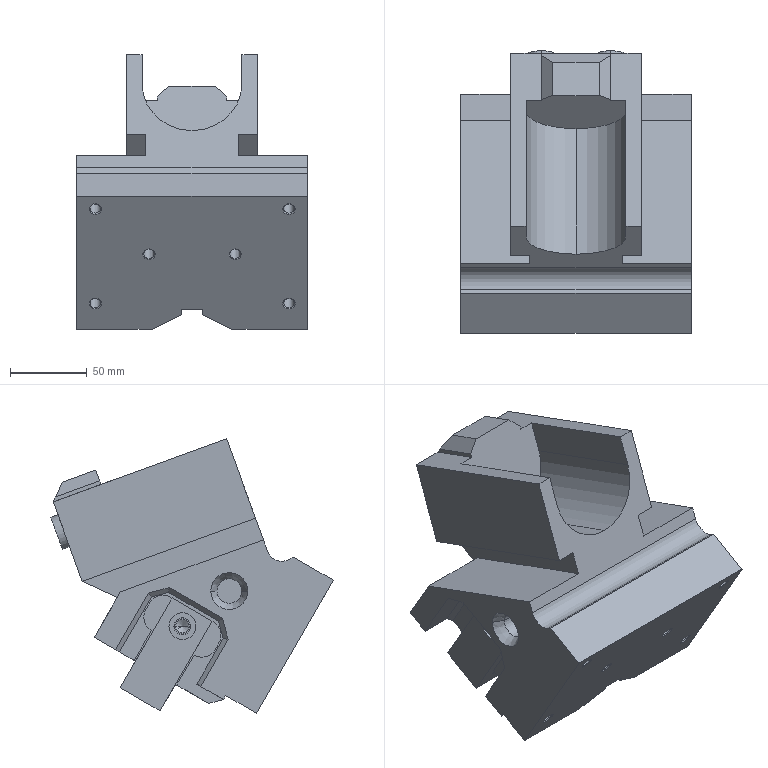Part | NX | features MEVN150-30_2;MEVN150-30_ASM|NEXT ASSEMBLY RELATIONSHIP#MGFV150-30_ASM|NEXT ASSEMBLY RELATIONSHIP#CAMSLIDER;CAMSLIDER 2 | 1 solid | 185 faces | box 150 x 183.756 x 178.57 mm | volume 1650795 mm3 | plane 118 | cylinder 47 | cone 20 | commonest cylinder face diameters 20 x13 6.8 x6 8.6 x4 10 x4 11 x4 16 x4